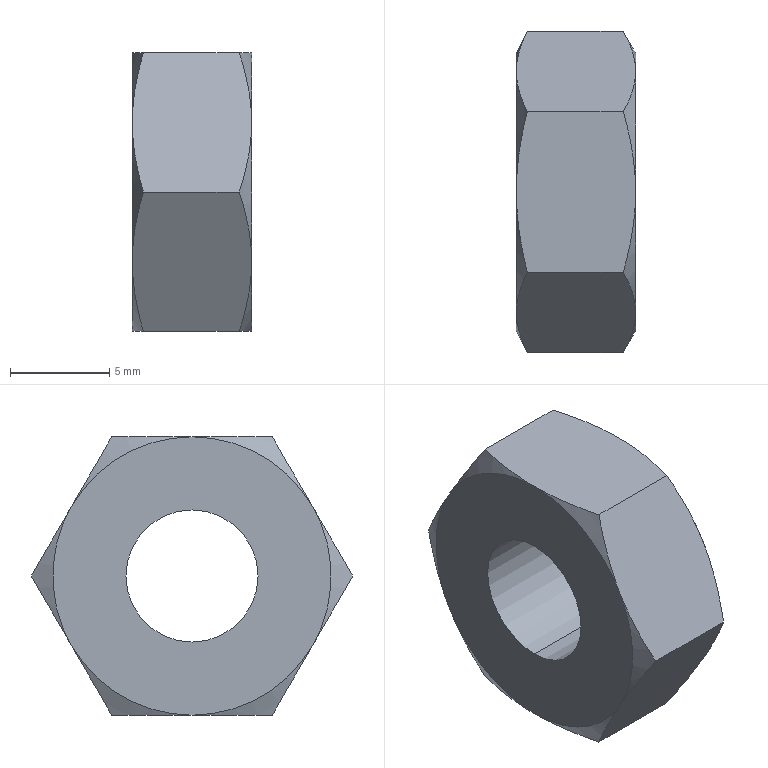Part | 1 solid | 22 faces | box 6 x 16.166 x 14 mm | volume 804.447 mm3 | cone 12 | plane 8 | cylinder 2 | commonest cylinder face diameters 6.647 x2
STEP:
#1=CARTESIAN_POINT('',(0.,0.,3.324));
#2=VERTEX_POINT('',#1);
#3=CARTESIAN_POINT('',(0.,0.,-3.324));
#4=VERTEX_POINT('',#3);
#5=CARTESIAN_POINT('',(0.,0.,0.));
#6=DIRECTION('',(1.,0.,0.));
#7=DIRECTION('',(0.,0.,-1.));
#8=AXIS2_PLACEMENT_3D('',#5,#6,#7);
#9=CIRCLE('',#8,3.324);
#10=EDGE_CURVE('',#2,#4,#9,.T.);
#11=ORIENTED_EDGE('',*,*,#10,.F.);
#12=CARTESIAN_POINT('',(6.,0.,3.324));
#13=VERTEX_POINT('',#12);
#14=CARTESIAN_POINT('',(6.,0.,3.324));
#15=DIRECTION('',(1.,0.,0.));
#16=VECTOR('',#15,1000.);
#17=LINE('',#14,#16);
#18=EDGE_CURVE('',#2,#13,#17,.T.);
#19=ORIENTED_EDGE('',*,*,#18,.T.);
#20=CARTESIAN_POINT('',(6.,0.,-3.324));
#21=VERTEX_POINT('',#20);
#22=CARTESIAN_POINT('',(6.,0.,0.));
#23=DIRECTION('',(1.,0.,0.));
#24=DIRECTION('',(0.,0.,-1.));
#25=AXIS2_PLACEMENT_3D('',#22,#23,#24);
#26=CIRCLE('',#25,3.324);
#27=EDGE_CURVE('',#13,#21,#26,.T.);
#28=ORIENTED_EDGE('',*,*,#27,.T.);
#29=CARTESIAN_POINT('',(6.,0.,-3.324));
#30=DIRECTION('',(1.,0.,0.));
#31=VECTOR('',#30,1000.);
#32=LINE('',#29,#31);
#33=EDGE_CURVE('',#4,#21,#32,.T.);
#34=ORIENTED_EDGE('',*,*,#33,.F.);
#35=EDGE_LOOP('',(#11,#19,#28,#34));
#36=FACE_OUTER_BOUND('',#35,.T.);
#37=CARTESIAN_POINT('',(6.,0.,0.));
#38=DIRECTION('',(1.,0.,0.));
#39=DIRECTION('',(0.,0.,-1.));
#40=AXIS2_PLACEMENT_3D('',#37,#38,#39);
#41=CYLINDRICAL_SURFACE('',#40,3.324);
#42=ADVANCED_FACE('',(#36),#41,.F.);
#43=CARTESIAN_POINT('',(5.375,-4.041,7.));
#44=VERTEX_POINT('',#43);
#45=CARTESIAN_POINT('',(6.,0.,7.));
#46=VERTEX_POINT('',#45);
#47=CARTESIAN_POINT('',(5.375,-4.041,7.));
#48=CARTESIAN_POINT('',(5.792,-2.598,7.));
#49=CARTESIAN_POINT('',(6.,-1.25,7.));
#50=CARTESIAN_POINT('',(6.,0.,7.));
#51=B_SPLINE_CURVE_WITH_KNOTS('',3,(#47,#48,#49,#50),.UNSPECIFIED.,.F.,.F.,(4,4),(0.,1.),.UNSPECIFIED.);
#52=EDGE_CURVE('',#44,#46,#51,.T.);
#53=ORIENTED_EDGE('',*,*,#52,.F.);
#54=CARTESIAN_POINT('',(6.,-6.062,3.5));
#55=VERTEX_POINT('',#54);
#56=CARTESIAN_POINT('',(6.,-6.062,3.5));
#57=CARTESIAN_POINT('',(6.,-5.437,4.583));
#58=CARTESIAN_POINT('',(5.792,-4.763,5.75));
#59=CARTESIAN_POINT('',(5.375,-4.041,7.));
#60=B_SPLINE_CURVE_WITH_KNOTS('',3,(#56,#57,#58,#59),.UNSPECIFIED.,.F.,.F.,(4,4),(0.,1.),.UNSPECIFIED.);
#61=EDGE_CURVE('',#55,#44,#60,.T.);
#62=ORIENTED_EDGE('',*,*,#61,.F.);
#63=CARTESIAN_POINT('',(6.,0.,0.));
#64=DIRECTION('',(1.,0.,0.));
#65=DIRECTION('',(0.,0.,-1.));
#66=AXIS2_PLACEMENT_3D('',#63,#64,#65);
#67=CIRCLE('',#66,7.);
#68=EDGE_CURVE('',#46,#55,#67,.T.);
#69=ORIENTED_EDGE('',*,*,#68,.F.);
#70=EDGE_LOOP('',(#53,#62,#69));
#71=FACE_OUTER_BOUND('',#70,.T.);
#72=CARTESIAN_POINT('',(6.,0.,0.));
#73=DIRECTION('',(-1.,0.,0.));
#74=DIRECTION('',(0.,0.,1.));
#75=AXIS2_PLACEMENT_3D('',#72,#73,#74);
#76=CONICAL_SURFACE('',#75,7.,1.047);
#77=ADVANCED_FACE('',(#71),#76,.T.);
#78=CARTESIAN_POINT('',(5.375,4.041,7.));
#79=VERTEX_POINT('',#78);
#80=CARTESIAN_POINT('',(6.,0.,7.));
#81=CARTESIAN_POINT('',(6.,1.25,7.));
#82=CARTESIAN_POINT('',(5.792,2.598,7.));
#83=CARTESIAN_POINT('',(5.375,4.041,7.));
#84=B_SPLINE_CURVE_WITH_KNOTS('',3,(#80,#81,#82,#83),.UNSPECIFIED.,.F.,.F.,(4,4),(0.,1.),.UNSPECIFIED.);
#85=EDGE_CURVE('',#46,#79,#84,.T.);
#86=ORIENTED_EDGE('',*,*,#85,.F.);
#87=CARTESIAN_POINT('',(6.,6.062,3.5));
#88=VERTEX_POINT('',#87);
#89=CARTESIAN_POINT('',(6.,0.,0.));
#90=DIRECTION('',(1.,0.,0.));
#91=DIRECTION('',(0.,0.,-1.));
#92=AXIS2_PLACEMENT_3D('',#89,#90,#91);
#93=CIRCLE('',#92,7.);
#94=EDGE_CURVE('',#88,#46,#93,.T.);
#95=ORIENTED_EDGE('',*,*,#94,.F.);
#96=CARTESIAN_POINT('',(5.375,4.041,7.));
#97=CARTESIAN_POINT('',(5.792,4.763,5.75));
#98=CARTESIAN_POINT('',(6.,5.437,4.583));
#99=CARTESIAN_POINT('',(6.,6.062,3.5));
#100=B_SPLINE_CURVE_WITH_KNOTS('',3,(#96,#97,#98,#99),.UNSPECIFIED.,.F.,.F.,(4,4),(0.,1.),.UNSPECIFIED.);
#101=EDGE_CURVE('',#79,#88,#100,.T.);
#102=ORIENTED_EDGE('',*,*,#101,.F.);
#103=EDGE_LOOP('',(#86,#95,#102));
#104=FACE_OUTER_BOUND('',#103,.T.);
#105=CARTESIAN_POINT('',(6.,0.,0.));
#106=DIRECTION('',(-1.,0.,0.));
#107=DIRECTION('',(0.,0.,1.));
#108=AXIS2_PLACEMENT_3D('',#105,#106,#107);
#109=CONICAL_SURFACE('',#108,7.,1.047);
#110=ADVANCED_FACE('',(#104),#109,.T.);
#111=CARTESIAN_POINT('',(5.375,8.083,0.));
#112=VERTEX_POINT('',#111);
#113=CARTESIAN_POINT('',(6.,6.062,3.5));
#114=CARTESIAN_POINT('',(6.,6.687,2.417));
#115=CARTESIAN_POINT('',(5.792,7.361,1.25));
#116=CARTESIAN_POINT('',(5.375,8.083,0.));
#117=B_SPLINE_CURVE_WITH_KNOTS('',3,(#113,#114,#115,#116),.UNSPECIFIED.,.F.,.F.,(4,4),(0.,1.),.UNSPECIFIED.);
#118=EDGE_CURVE('',#88,#112,#117,.T.);
#119=ORIENTED_EDGE('',*,*,#118,.F.);
#120=CARTESIAN_POINT('',(6.,6.062,-3.5));
#121=VERTEX_POINT('',#120);
#122=CARTESIAN_POINT('',(6.,0.,0.));
#123=DIRECTION('',(1.,0.,0.));
#124=DIRECTION('',(0.,0.,-1.));
#125=AXIS2_PLACEMENT_3D('',#122,#123,#124);
#126=CIRCLE('',#125,7.);
#127=EDGE_CURVE('',#121,#88,#126,.T.);
#128=ORIENTED_EDGE('',*,*,#127,.F.);
#129=CARTESIAN_POINT('',(5.375,8.083,0.));
#130=CARTESIAN_POINT('',(5.792,7.361,-1.25));
#131=CARTESIAN_POINT('',(6.,6.687,-2.417));
#132=CARTESIAN_POINT('',(6.,6.062,-3.5));
#133=B_SPLINE_CURVE_WITH_KNOTS('',3,(#129,#130,#131,#132),.UNSPECIFIED.,.F.,.F.,(4,4),(0.,1.),.UNSPECIFIED.);
#134=EDGE_CURVE('',#112,#121,#133,.T.);
#135=ORIENTED_EDGE('',*,*,#134,.F.);
#136=EDGE_LOOP('',(#119,#128,#135));
#137=FACE_OUTER_BOUND('',#136,.T.);
#138=CARTESIAN_POINT('',(6.,0.,0.));
#139=DIRECTION('',(-1.,0.,0.));
#140=DIRECTION('',(0.,0.,1.));
#141=AXIS2_PLACEMENT_3D('',#138,#139,#140);
#142=CONICAL_SURFACE('',#141,7.,1.047);
#143=ADVANCED_FACE('',(#137),#142,.T.);
#144=CARTESIAN_POINT('',(5.375,4.041,-7.));
#145=VERTEX_POINT('',#144);
#146=CARTESIAN_POINT('',(6.,6.062,-3.5));
#147=CARTESIAN_POINT('',(6.,5.437,-4.583));
#148=CARTESIAN_POINT('',(5.792,4.763,-5.75));
#149=CARTESIAN_POINT('',(5.375,4.041,-7.));
#150=B_SPLINE_CURVE_WITH_KNOTS('',3,(#146,#147,#148,#149),.UNSPECIFIED.,.F.,.F.,(4,4),(0.,1.),.UNSPECIFIED.);
#151=EDGE_CURVE('',#121,#145,#150,.T.);
#152=ORIENTED_EDGE('',*,*,#151,.F.);
#153=CARTESIAN_POINT('',(6.,0.,-7.));
#154=VERTEX_POINT('',#153);
#155=CARTESIAN_POINT('',(6.,0.,0.));
#156=DIRECTION('',(1.,0.,0.));
#157=DIRECTION('',(0.,0.,-1.));
#158=AXIS2_PLACEMENT_3D('',#155,#156,#157);
#159=CIRCLE('',#158,7.);
#160=EDGE_CURVE('',#154,#121,#159,.T.);
#161=ORIENTED_EDGE('',*,*,#160,.F.);
#162=CARTESIAN_POINT('',(5.375,4.041,-7.));
#163=CARTESIAN_POINT('',(5.792,2.598,-7.));
#164=CARTESIAN_POINT('',(6.,1.25,-7.));
#165=CARTESIAN_POINT('',(6.,0.,-7.));
#166=B_SPLINE_CURVE_WITH_KNOTS('',3,(#162,#163,#164,#165),.UNSPECIFIED.,.F.,.F.,(4,4),(0.,1.),.UNSPECIFIED.);
#167=EDGE_CURVE('',#145,#154,#166,.T.);
#168=ORIENTED_EDGE('',*,*,#167,.F.);
#169=EDGE_LOOP('',(#152,#161,#168));
#170=FACE_OUTER_BOUND('',#169,.T.);
#171=CARTESIAN_POINT('',(6.,0.,0.));
#172=DIRECTION('',(-1.,0.,0.));
#173=DIRECTION('',(0.,0.,1.));
#174=AXIS2_PLACEMENT_3D('',#171,#172,#173);
#175=CONICAL_SURFACE('',#174,7.,1.047);
#176=ADVANCED_FACE('',(#170),#175,.T.);
#177=CARTESIAN_POINT('',(5.375,-4.041,-7.));
#178=VERTEX_POINT('',#177);
#179=CARTESIAN_POINT('',(6.,0.,-7.));
#180=CARTESIAN_POINT('',(6.,-1.25,-7.));
#181=CARTESIAN_POINT('',(5.792,-2.598,-7.));
#182=CARTESIAN_POINT('',(5.375,-4.041,-7.));
#183=B_SPLINE_CURVE_WITH_KNOTS('',3,(#179,#180,#181,#182),.UNSPECIFIED.,.F.,.F.,(4,4),(0.,1.),.UNSPECIFIED.);
#184=EDGE_CURVE('',#154,#178,#183,.T.);
#185=ORIENTED_EDGE('',*,*,#184,.F.);
#186=CARTESIAN_POINT('',(6.,-6.062,-3.5));
#187=VERTEX_POINT('',#186);
#188=CARTESIAN_POINT('',(6.,0.,0.));
#189=DIRECTION('',(1.,0.,0.));
#190=DIRECTION('',(0.,0.,-1.));
#191=AXIS2_PLACEMENT_3D('',#188,#189,#190);
#192=CIRCLE('',#191,7.);
#193=EDGE_CURVE('',#187,#154,#192,.T.);
#194=ORIENTED_EDGE('',*,*,#193,.F.);
#195=CARTESIAN_POINT('',(5.375,-4.041,-7.));
#196=CARTESIAN_POINT('',(5.792,-4.763,-5.75));
#197=CARTESIAN_POINT('',(6.,-5.437,-4.583));
#198=CARTESIAN_POINT('',(6.,-6.062,-3.5));
#199=B_SPLINE_CURVE_WITH_KNOTS('',3,(#195,#196,#197,#198),.UNSPECIFIED.,.F.,.F.,(4,4),(0.,1.),.UNSPECIFIED.);
#200=EDGE_CURVE('',#178,#187,#199,.T.);
#201=ORIENTED_EDGE('',*,*,#200,.F.);
#202=EDGE_LOOP('',(#185,#194,#201));
#203=FACE_OUTER_BOUND('',#202,.T.);
#204=CARTESIAN_POINT('',(6.,0.,0.));
#205=DIRECTION('',(-1.,0.,0.));
#206=DIRECTION('',(0.,0.,1.));
#207=AXIS2_PLACEMENT_3D('',#204,#205,#206);
#208=CONICAL_SURFACE('',#207,7.,1.047);
#209=ADVANCED_FACE('',(#203),#208,.T.);
#210=CARTESIAN_POINT('',(0.5518,4.041,-7.));
#211=VERTEX_POINT('',#210);
#212=CARTESIAN_POINT('',(0.,6.062,-3.5));
#213=VERTEX_POINT('',#212);
#214=CARTESIAN_POINT('',(0.5518,4.041,-7.));
#215=CARTESIAN_POINT('',(0.1839,4.763,-5.75));
#216=CARTESIAN_POINT('',(0.,5.437,-4.583));
#217=CARTESIAN_POINT('',(0.,6.062,-3.5));
#218=B_SPLINE_CURVE_WITH_KNOTS('',3,(#214,#215,#216,#217),.UNSPECIFIED.,.F.,.F.,(4,4),(0.,1.),.UNSPECIFIED.);
#219=EDGE_CURVE('',#211,#213,#218,.T.);
#220=ORIENTED_EDGE('',*,*,#219,.F.);
#221=CARTESIAN_POINT('',(0.,0.,-7.));
#222=VERTEX_POINT('',#221);
#223=CARTESIAN_POINT('',(0.,0.,-7.));
#224=CARTESIAN_POINT('',(0.,1.25,-7.));
#225=CARTESIAN_POINT('',(0.1839,2.598,-7.));
#226=CARTESIAN_POINT('',(0.5518,4.041,-7.));
#227=B_SPLINE_CURVE_WITH_KNOTS('',3,(#223,#224,#225,#226),.UNSPECIFIED.,.F.,.F.,(4,4),(0.,1.),.UNSPECIFIED.);
#228=EDGE_CURVE('',#222,#211,#227,.T.);
#229=ORIENTED_EDGE('',*,*,#228,.F.);
#230=CARTESIAN_POINT('',(0.,0.,0.));
#231=DIRECTION('',(1.,0.,0.));
#232=DIRECTION('',(0.,0.,-1.));
#233=AXIS2_PLACEMENT_3D('',#230,#231,#232);
#234=CIRCLE('',#233,7.);
#235=EDGE_CURVE('',#222,#213,#234,.T.);
#236=ORIENTED_EDGE('',*,*,#235,.T.);
#237=EDGE_LOOP('',(#220,#229,#236));
#238=FACE_OUTER_BOUND('',#237,.T.);
#239=CARTESIAN_POINT('',(2.813,0.,0.));
#240=DIRECTION('',(1.,0.,0.));
#241=DIRECTION('',(0.,0.,-1.));
#242=AXIS2_PLACEMENT_3D('',#239,#240,#241);
#243=CONICAL_SURFACE('',#242,12.52,1.1);
#244=ADVANCED_FACE('',(#238),#243,.T.);
#245=CARTESIAN_POINT('',(0.5518,8.083,0.));
#246=VERTEX_POINT('',#245);
#247=CARTESIAN_POINT('',(0.,6.062,-3.5));
#248=CARTESIAN_POINT('',(0.,6.687,-2.417));
#249=CARTESIAN_POINT('',(0.1839,7.361,-1.25));
#250=CARTESIAN_POINT('',(0.5518,8.083,0.));
#251=B_SPLINE_CURVE_WITH_KNOTS('',3,(#247,#248,#249,#250),.UNSPECIFIED.,.F.,.F.,(4,4),(0.,1.),.UNSPECIFIED.);
#252=EDGE_CURVE('',#213,#246,#251,.T.);
#253=ORIENTED_EDGE('',*,*,#252,.F.);
#254=CARTESIAN_POINT('',(0.,6.062,3.5));
#255=VERTEX_POINT('',#254);
#256=CARTESIAN_POINT('',(0.,0.,0.));
#257=DIRECTION('',(1.,0.,0.));
#258=DIRECTION('',(0.,0.,-1.));
#259=AXIS2_PLACEMENT_3D('',#256,#257,#258);
#260=CIRCLE('',#259,7.);
#261=EDGE_CURVE('',#213,#255,#260,.T.);
#262=ORIENTED_EDGE('',*,*,#261,.T.);
#263=CARTESIAN_POINT('',(0.5518,8.083,0.));
#264=CARTESIAN_POINT('',(0.1839,7.361,1.25));
#265=CARTESIAN_POINT('',(0.,6.687,2.417));
#266=CARTESIAN_POINT('',(0.,6.062,3.5));
#267=B_SPLINE_CURVE_WITH_KNOTS('',3,(#263,#264,#265,#266),.UNSPECIFIED.,.F.,.F.,(4,4),(0.,1.),.UNSPECIFIED.);
#268=EDGE_CURVE('',#246,#255,#267,.T.);
#269=ORIENTED_EDGE('',*,*,#268,.F.);
#270=EDGE_LOOP('',(#253,#262,#269));
#271=FACE_OUTER_BOUND('',#270,.T.);
#272=CARTESIAN_POINT('',(2.813,0.,0.));
#273=DIRECTION('',(1.,0.,0.));
#274=DIRECTION('',(0.,0.,-1.));
#275=AXIS2_PLACEMENT_3D('',#272,#273,#274);
#276=CONICAL_SURFACE('',#275,12.52,1.1);
#277=ADVANCED_FACE('',(#271),#276,.T.);
#278=CARTESIAN_POINT('',(0.5518,4.041,7.));
#279=VERTEX_POINT('',#278);
#280=CARTESIAN_POINT('',(0.,6.062,3.5));
#281=CARTESIAN_POINT('',(0.,5.437,4.583));
#282=CARTESIAN_POINT('',(0.1839,4.763,5.75));
#283=CARTESIAN_POINT('',(0.5518,4.041,7.));
#284=B_SPLINE_CURVE_WITH_KNOTS('',3,(#280,#281,#282,#283),.UNSPECIFIED.,.F.,.F.,(4,4),(0.,1.),.UNSPECIFIED.);
#285=EDGE_CURVE('',#255,#279,#284,.T.);
#286=ORIENTED_EDGE('',*,*,#285,.F.);
#287=CARTESIAN_POINT('',(0.,0.,7.));
#288=VERTEX_POINT('',#287);
#289=CARTESIAN_POINT('',(0.,0.,0.));
#290=DIRECTION('',(1.,0.,0.));
#291=DIRECTION('',(0.,0.,-1.));
#292=AXIS2_PLACEMENT_3D('',#289,#290,#291);
#293=CIRCLE('',#292,7.);
#294=EDGE_CURVE('',#255,#288,#293,.T.);
#295=ORIENTED_EDGE('',*,*,#294,.T.);
#296=CARTESIAN_POINT('',(0.5518,4.041,7.));
#297=CARTESIAN_POINT('',(0.1839,2.598,7.));
#298=CARTESIAN_POINT('',(0.,1.25,7.));
#299=CARTESIAN_POINT('',(0.,0.,7.));
#300=B_SPLINE_CURVE_WITH_KNOTS('',3,(#296,#297,#298,#299),.UNSPECIFIED.,.F.,.F.,(4,4),(0.,1.),.UNSPECIFIED.);
#301=EDGE_CURVE('',#279,#288,#300,.T.);
#302=ORIENTED_EDGE('',*,*,#301,.F.);
#303=EDGE_LOOP('',(#286,#295,#302));
#304=FACE_OUTER_BOUND('',#303,.T.);
#305=CARTESIAN_POINT('',(2.813,0.,0.));
#306=DIRECTION('',(1.,0.,0.));
#307=DIRECTION('',(0.,0.,-1.));
#308=AXIS2_PLACEMENT_3D('',#305,#306,#307);
#309=CONICAL_SURFACE('',#308,12.52,1.1);
#310=ADVANCED_FACE('',(#304),#309,.T.);
#311=CARTESIAN_POINT('',(0.5518,-4.041,-7.));
#312=VERTEX_POINT('',#311);
#313=CARTESIAN_POINT('',(0.5518,-4.041,-7.));
#314=CARTESIAN_POINT('',(0.1839,-2.598,-7.));
#315=CARTESIAN_POINT('',(0.,-1.25,-7.));
#316=CARTESIAN_POINT('',(0.,0.,-7.));
#317=B_SPLINE_CURVE_WITH_KNOTS('',3,(#313,#314,#315,#316),.UNSPECIFIED.,.F.,.F.,(4,4),(0.,1.),.UNSPECIFIED.);
#318=EDGE_CURVE('',#312,#222,#317,.T.);
#319=ORIENTED_EDGE('',*,*,#318,.F.);
#320=CARTESIAN_POINT('',(0.,-6.062,-3.5));
#321=VERTEX_POINT('',#320);
#322=CARTESIAN_POINT('',(0.,-6.062,-3.5));
#323=CARTESIAN_POINT('',(0.,-5.437,-4.583));
#324=CARTESIAN_POINT('',(0.1839,-4.763,-5.75));
#325=CARTESIAN_POINT('',(0.5518,-4.041,-7.));
#326=B_SPLINE_CURVE_WITH_KNOTS('',3,(#322,#323,#324,#325),.UNSPECIFIED.,.F.,.F.,(4,4),(0.,1.),.UNSPECIFIED.);
#327=EDGE_CURVE('',#321,#312,#326,.T.);
#328=ORIENTED_EDGE('',*,*,#327,.F.);
#329=CARTESIAN_POINT('',(0.,0.,0.));
#330=DIRECTION('',(1.,0.,0.));
#331=DIRECTION('',(0.,0.,-1.));
#332=AXIS2_PLACEMENT_3D('',#329,#330,#331);
#333=CIRCLE('',#332,7.);
#334=EDGE_CURVE('',#321,#222,#333,.T.);
#335=ORIENTED_EDGE('',*,*,#334,.T.);
#336=EDGE_LOOP('',(#319,#328,#335));
#337=FACE_OUTER_BOUND('',#336,.T.);
#338=CARTESIAN_POINT('',(2.813,0.,0.));
#339=DIRECTION('',(1.,0.,0.));
#340=DIRECTION('',(0.,0.,-1.));
#341=AXIS2_PLACEMENT_3D('',#338,#339,#340);
#342=CONICAL_SURFACE('',#341,12.52,1.1);
#343=ADVANCED_FACE('',(#337),#342,.T.);
#344=CARTESIAN_POINT('',(0.5518,-4.041,7.));
#345=VERTEX_POINT('',#344);
#346=CARTESIAN_POINT('',(0.,0.,7.));
#347=CARTESIAN_POINT('',(0.,-1.25,7.));
#348=CARTESIAN_POINT('',(0.1839,-2.598,7.));
#349=CARTESIAN_POINT('',(0.5518,-4.041,7.));
#350=B_SPLINE_CURVE_WITH_KNOTS('',3,(#346,#347,#348,#349),.UNSPECIFIED.,.F.,.F.,(4,4),(0.,1.),.UNSPECIFIED.);
#351=EDGE_CURVE('',#288,#345,#350,.T.);
#352=ORIENTED_EDGE('',*,*,#351,.F.);
#353=CARTESIAN_POINT('',(0.,-6.062,3.5));
#354=VERTEX_POINT('',#353);
#355=CARTESIAN_POINT('',(0.,0.,0.));
#356=DIRECTION('',(1.,0.,0.));
#357=DIRECTION('',(0.,0.,-1.));
#358=AXIS2_PLACEMENT_3D('',#355,#356,#357);
#359=CIRCLE('',#358,7.);
#360=EDGE_CURVE('',#288,#354,#359,.T.);
#361=ORIENTED_EDGE('',*,*,#360,.T.);
#362=CARTESIAN_POINT('',(0.5518,-4.041,7.));
#363=CARTESIAN_POINT('',(0.1839,-4.763,5.75));
#364=CARTESIAN_POINT('',(0.,-5.437,4.583));
#365=CARTESIAN_POINT('',(0.,-6.062,3.5));
#366=B_SPLINE_CURVE_WITH_KNOTS('',3,(#362,#363,#364,#365),.UNSPECIFIED.,.F.,.F.,(4,4),(0.,1.),.UNSPECIFIED.);
#367=EDGE_CURVE('',#345,#354,#366,.T.);
#368=ORIENTED_EDGE('',*,*,#367,.F.);
#369=EDGE_LOOP('',(#352,#361,#368));
#370=FACE_OUTER_BOUND('',#369,.T.);
#371=CARTESIAN_POINT('',(2.813,0.,0.));
#372=DIRECTION('',(1.,0.,0.));
#373=DIRECTION('',(0.,0.,-1.));
#374=AXIS2_PLACEMENT_3D('',#371,#372,#373);
#375=CONICAL_SURFACE('',#374,12.52,1.1);
#376=ADVANCED_FACE('',(#370),#375,.T.);
#377=CARTESIAN_POINT('',(0.,0.,0.));
#378=DIRECTION('',(1.,0.,0.));
#379=DIRECTION('',(0.,0.,-1.));
#380=AXIS2_PLACEMENT_3D('',#377,#378,#379);
#381=CIRCLE('',#380,3.324);
#382=EDGE_CURVE('',#4,#2,#381,.T.);
#383=ORIENTED_EDGE('',*,*,#382,.T.);
#384=ORIENTED_EDGE('',*,*,#10,.T.);
#385=EDGE_LOOP('',(#383,#384));
#386=FACE_BOUND('',#385,.T.);
#387=ORIENTED_EDGE('',*,*,#235,.F.);
#388=ORIENTED_EDGE('',*,*,#334,.F.);
#389=CARTESIAN_POINT('',(0.,0.,0.));
#390=DIRECTION('',(1.,0.,0.));
#391=DIRECTION('',(0.,0.,-1.));
#392=AXIS2_PLACEMENT_3D('',#389,#390,#391);
#393=CIRCLE('',#392,7.);
#394=EDGE_CURVE('',#354,#321,#393,.T.);
#395=ORIENTED_EDGE('',*,*,#394,.F.);
#396=ORIENTED_EDGE('',*,*,#360,.F.);
#397=ORIENTED_EDGE('',*,*,#294,.F.);
#398=ORIENTED_EDGE('',*,*,#261,.F.);
#399=EDGE_LOOP('',(#387,#388,#395,#396,#397,#398));
#400=FACE_OUTER_BOUND('',#399,.T.);
#401=CARTESIAN_POINT('',(0.,7.,0.));
#402=DIRECTION('',(-1.,0.,0.));
#403=DIRECTION('',(0.,0.,1.));
#404=AXIS2_PLACEMENT_3D('',#401,#402,#403);
#405=PLANE('',#404);
#406=ADVANCED_FACE('',(#386,#400),#405,.T.);
#407=ORIENTED_EDGE('',*,*,#18,.F.);
#408=ORIENTED_EDGE('',*,*,#382,.F.);
#409=ORIENTED_EDGE('',*,*,#33,.T.);
#410=CARTESIAN_POINT('',(6.,0.,0.));
#411=DIRECTION('',(1.,0.,0.));
#412=DIRECTION('',(0.,0.,-1.));
#413=AXIS2_PLACEMENT_3D('',#410,#411,#412);
#414=CIRCLE('',#413,3.324);
#415=EDGE_CURVE('',#21,#13,#414,.T.);
#416=ORIENTED_EDGE('',*,*,#415,.T.);
#417=EDGE_LOOP('',(#407,#408,#409,#416));
#418=FACE_OUTER_BOUND('',#417,.T.);
#419=CARTESIAN_POINT('',(6.,0.,0.));
#420=DIRECTION('',(1.,0.,0.));
#421=DIRECTION('',(0.,0.,-1.));
#422=AXIS2_PLACEMENT_3D('',#419,#420,#421);
#423=CYLINDRICAL_SURFACE('',#422,3.324);
#424=ADVANCED_FACE('',(#418),#423,.F.);
#425=ORIENTED_EDGE('',*,*,#160,.T.);
#426=ORIENTED_EDGE('',*,*,#127,.T.);
#427=ORIENTED_EDGE('',*,*,#94,.T.);
#428=ORIENTED_EDGE('',*,*,#68,.T.);
#429=CARTESIAN_POINT('',(6.,0.,0.));
#430=DIRECTION('',(1.,0.,0.));
#431=DIRECTION('',(0.,0.,-1.));
#432=AXIS2_PLACEMENT_3D('',#429,#430,#431);
#433=CIRCLE('',#432,7.);
#434=EDGE_CURVE('',#55,#187,#433,.T.);
#435=ORIENTED_EDGE('',*,*,#434,.T.);
#436=ORIENTED_EDGE('',*,*,#193,.T.);
#437=EDGE_LOOP('',(#425,#426,#427,#428,#435,#436));
#438=FACE_OUTER_BOUND('',#437,.T.);
#439=ORIENTED_EDGE('',*,*,#415,.F.);
#440=ORIENTED_EDGE('',*,*,#27,.F.);
#441=EDGE_LOOP('',(#439,#440));
#442=FACE_BOUND('',#441,.T.);
#443=CARTESIAN_POINT('',(6.,3.324,0.));
#444=DIRECTION('',(1.,0.,0.));
#445=DIRECTION('',(0.,1.,0.));
#446=AXIS2_PLACEMENT_3D('',#443,#444,#445);
#447=PLANE('',#446);
#448=ADVANCED_FACE('',(#438,#442),#447,.T.);
#449=CARTESIAN_POINT('',(5.375,-8.083,0.));
#450=VERTEX_POINT('',#449);
#451=CARTESIAN_POINT('',(6.,-6.062,-3.5));
#452=CARTESIAN_POINT('',(6.,-6.687,-2.417));
#453=CARTESIAN_POINT('',(5.792,-7.361,-1.25));
#454=CARTESIAN_POINT('',(5.375,-8.083,0.));
#455=B_SPLINE_CURVE_WITH_KNOTS('',3,(#451,#452,#453,#454),.UNSPECIFIED.,.F.,.F.,(4,4),(0.,1.),.UNSPECIFIED.);
#456=EDGE_CURVE('',#187,#450,#455,.T.);
#457=ORIENTED_EDGE('',*,*,#456,.F.);
#458=ORIENTED_EDGE('',*,*,#434,.F.);
#459=CARTESIAN_POINT('',(5.375,-8.083,0.));
#460=CARTESIAN_POINT('',(5.792,-7.361,1.25));
#461=CARTESIAN_POINT('',(6.,-6.687,2.417));
#462=CARTESIAN_POINT('',(6.,-6.062,3.5));
#463=B_SPLINE_CURVE_WITH_KNOTS('',3,(#459,#460,#461,#462),.UNSPECIFIED.,.F.,.F.,(4,4),(0.,1.),.UNSPECIFIED.);
#464=EDGE_CURVE('',#450,#55,#463,.T.);
#465=ORIENTED_EDGE('',*,*,#464,.F.);
#466=EDGE_LOOP('',(#457,#458,#465));
#467=FACE_OUTER_BOUND('',#466,.T.);
#468=CARTESIAN_POINT('',(6.,0.,0.));
#469=DIRECTION('',(-1.,0.,0.));
#470=DIRECTION('',(0.,0.,1.));
#471=AXIS2_PLACEMENT_3D('',#468,#469,#470);
#472=CONICAL_SURFACE('',#471,7.,1.047);
#473=ADVANCED_FACE('',(#467),#472,.T.);
#474=CARTESIAN_POINT('',(0.5518,-8.083,0.));
#475=VERTEX_POINT('',#474);
#476=CARTESIAN_POINT('',(0.5518,-8.083,0.));
#477=CARTESIAN_POINT('',(0.1839,-7.361,-1.25));
#478=CARTESIAN_POINT('',(0.,-6.687,-2.417));
#479=CARTESIAN_POINT('',(0.,-6.062,-3.5));
#480=B_SPLINE_CURVE_WITH_KNOTS('',3,(#476,#477,#478,#479),.UNSPECIFIED.,.F.,.F.,(4,4),(0.,1.),.UNSPECIFIED.);
#481=EDGE_CURVE('',#475,#321,#480,.T.);
#482=ORIENTED_EDGE('',*,*,#481,.F.);
#483=CARTESIAN_POINT('',(0.,-6.062,3.5));
#484=CARTESIAN_POINT('',(0.,-6.687,2.417));
#485=CARTESIAN_POINT('',(0.1839,-7.361,1.25));
#486=CARTESIAN_POINT('',(0.5518,-8.083,0.));
#487=B_SPLINE_CURVE_WITH_KNOTS('',3,(#483,#484,#485,#486),.UNSPECIFIED.,.F.,.F.,(4,4),(0.,1.),.UNSPECIFIED.);
#488=EDGE_CURVE('',#354,#475,#487,.T.);
#489=ORIENTED_EDGE('',*,*,#488,.F.);
#490=ORIENTED_EDGE('',*,*,#394,.T.);
#491=EDGE_LOOP('',(#482,#489,#490));
#492=FACE_OUTER_BOUND('',#491,.T.);
#493=CARTESIAN_POINT('',(2.813,0.,0.));
#494=DIRECTION('',(1.,0.,0.));
#495=DIRECTION('',(0.,0.,-1.));
#496=AXIS2_PLACEMENT_3D('',#493,#494,#495);
#497=CONICAL_SURFACE('',#496,12.52,1.1);
#498=ADVANCED_FACE('',(#492),#497,.T.);
#499=ORIENTED_EDGE('',*,*,#52,.T.);
#500=ORIENTED_EDGE('',*,*,#85,.T.);
#501=CARTESIAN_POINT('',(6.,4.041,7.));
#502=DIRECTION('',(-1.,0.,0.));
#503=VECTOR('',#502,1000.);
#504=LINE('',#501,#503);
#505=EDGE_CURVE('',#79,#279,#504,.T.);
#506=ORIENTED_EDGE('',*,*,#505,.T.);
#507=ORIENTED_EDGE('',*,*,#301,.T.);
#508=ORIENTED_EDGE('',*,*,#351,.T.);
#509=CARTESIAN_POINT('',(6.,-4.041,7.));
#510=DIRECTION('',(-1.,0.,0.));
#511=VECTOR('',#510,1000.);
#512=LINE('',#509,#511);
#513=EDGE_CURVE('',#44,#345,#512,.T.);
#514=ORIENTED_EDGE('',*,*,#513,.F.);
#515=EDGE_LOOP('',(#499,#500,#506,#507,#508,#514));
#516=FACE_OUTER_BOUND('',#515,.T.);
#517=CARTESIAN_POINT('',(6.,4.041,7.));
#518=DIRECTION('',(0.,0.,-1.));
#519=DIRECTION('',(0.,-1.,0.));
#520=AXIS2_PLACEMENT_3D('',#517,#518,#519);
#521=PLANE('',#520);
#522=ADVANCED_FACE('',(#516),#521,.F.);
#523=ORIENTED_EDGE('',*,*,#101,.T.);
#524=ORIENTED_EDGE('',*,*,#118,.T.);
#525=CARTESIAN_POINT('',(6.,8.083,0.));
#526=DIRECTION('',(-1.,0.,0.));
#527=VECTOR('',#526,1000.);
#528=LINE('',#525,#527);
#529=EDGE_CURVE('',#112,#246,#528,.T.);
#530=ORIENTED_EDGE('',*,*,#529,.T.);
#531=ORIENTED_EDGE('',*,*,#268,.T.);
#532=ORIENTED_EDGE('',*,*,#285,.T.);
#533=ORIENTED_EDGE('',*,*,#505,.F.);
#534=EDGE_LOOP('',(#523,#524,#530,#531,#532,#533));
#535=FACE_OUTER_BOUND('',#534,.T.);
#536=CARTESIAN_POINT('',(6.,8.083,0.));
#537=DIRECTION('',(0.,-0.866,-0.5));
#538=DIRECTION('',(0.,0.5,-0.866));
#539=AXIS2_PLACEMENT_3D('',#536,#537,#538);
#540=PLANE('',#539);
#541=ADVANCED_FACE('',(#535),#540,.F.);
#542=ORIENTED_EDGE('',*,*,#134,.T.);
#543=ORIENTED_EDGE('',*,*,#151,.T.);
#544=CARTESIAN_POINT('',(6.,4.041,-7.));
#545=DIRECTION('',(-1.,0.,0.));
#546=VECTOR('',#545,1000.);
#547=LINE('',#544,#546);
#548=EDGE_CURVE('',#145,#211,#547,.T.);
#549=ORIENTED_EDGE('',*,*,#548,.T.);
#550=ORIENTED_EDGE('',*,*,#219,.T.);
#551=ORIENTED_EDGE('',*,*,#252,.T.);
#552=ORIENTED_EDGE('',*,*,#529,.F.);
#553=EDGE_LOOP('',(#542,#543,#549,#550,#551,#552));
#554=FACE_OUTER_BOUND('',#553,.T.);
#555=CARTESIAN_POINT('',(6.,4.041,-7.));
#556=DIRECTION('',(0.,-0.866,0.5));
#557=DIRECTION('',(-1.,0.,0.));
#558=AXIS2_PLACEMENT_3D('',#555,#556,#557);
#559=PLANE('',#558);
#560=ADVANCED_FACE('',(#554),#559,.F.);
#561=ORIENTED_EDGE('',*,*,#167,.T.);
#562=ORIENTED_EDGE('',*,*,#184,.T.);
#563=CARTESIAN_POINT('',(6.,-4.041,-7.));
#564=DIRECTION('',(-1.,0.,0.));
#565=VECTOR('',#564,1000.);
#566=LINE('',#563,#565);
#567=EDGE_CURVE('',#178,#312,#566,.T.);
#568=ORIENTED_EDGE('',*,*,#567,.T.);
#569=ORIENTED_EDGE('',*,*,#318,.T.);
#570=ORIENTED_EDGE('',*,*,#228,.T.);
#571=ORIENTED_EDGE('',*,*,#548,.F.);
#572=EDGE_LOOP('',(#561,#562,#568,#569,#570,#571));
#573=FACE_OUTER_BOUND('',#572,.T.);
#574=CARTESIAN_POINT('',(6.,-4.041,-7.));
#575=DIRECTION('',(0.,0.,1.));
#576=DIRECTION('',(1.,0.,0.));
#577=AXIS2_PLACEMENT_3D('',#574,#575,#576);
#578=PLANE('',#577);
#579=ADVANCED_FACE('',(#573),#578,.F.);
#580=ORIENTED_EDGE('',*,*,#200,.T.);
#581=ORIENTED_EDGE('',*,*,#456,.T.);
#582=CARTESIAN_POINT('',(6.,-8.083,0.));
#583=DIRECTION('',(-1.,0.,0.));
#584=VECTOR('',#583,1000.);
#585=LINE('',#582,#584);
#586=EDGE_CURVE('',#450,#475,#585,.T.);
#587=ORIENTED_EDGE('',*,*,#586,.T.);
#588=ORIENTED_EDGE('',*,*,#481,.T.);
#589=ORIENTED_EDGE('',*,*,#327,.T.);
#590=ORIENTED_EDGE('',*,*,#567,.F.);
#591=EDGE_LOOP('',(#580,#581,#587,#588,#589,#590));
#592=FACE_OUTER_BOUND('',#591,.T.);
#593=CARTESIAN_POINT('',(6.,-8.083,0.));
#594=DIRECTION('',(0.,0.866,0.5));
#595=DIRECTION('',(1.,0.,0.));
#596=AXIS2_PLACEMENT_3D('',#593,#594,#595);
#597=PLANE('',#596);
#598=ADVANCED_FACE('',(#592),#597,.F.);
#599=ORIENTED_EDGE('',*,*,#464,.T.);
#600=ORIENTED_EDGE('',*,*,#61,.T.);
#601=ORIENTED_EDGE('',*,*,#513,.T.);
#602=ORIENTED_EDGE('',*,*,#367,.T.);
#603=ORIENTED_EDGE('',*,*,#488,.T.);
#604=ORIENTED_EDGE('',*,*,#586,.F.);
#605=EDGE_LOOP('',(#599,#600,#601,#602,#603,#604));
#606=FACE_OUTER_BOUND('',#605,.T.);
#607=CARTESIAN_POINT('',(6.,-4.041,7.));
#608=DIRECTION('',(0.,0.866,-0.5));
#609=DIRECTION('',(-1.,0.,0.));
#610=AXIS2_PLACEMENT_3D('',#607,#608,#609);
#611=PLANE('',#610);
#612=ADVANCED_FACE('',(#606),#611,.F.);
#613=CLOSED_SHELL('',(#42,#77,#110,#143,#176,#209,#244,#277,#310,#343,#376,#406,#424,#448,#473,#498,#522,#541,#560,#579,#598,#612));
#614=MANIFOLD_SOLID_BREP('',#613);
#615=CARTESIAN_POINT('',(0.,0.,0.));
#616=DIRECTION('',(0.,0.,1.));
#617=DIRECTION('',(1.,0.,0.));
#618=AXIS2_PLACEMENT_3D('',#615,#616,#617);
#619=(LENGTH_UNIT()NAMED_UNIT(*)SI_UNIT(.MILLI.,.METRE.));
#620=UNCERTAINTY_MEASURE_WITH_UNIT(LENGTH_MEASURE(0.00001),#619,'','');
#621=(NAMED_UNIT(*)PLANE_ANGLE_UNIT()SI_UNIT($,.RADIAN.));
#622=(NAMED_UNIT(*)SI_UNIT($,.STERADIAN.)SOLID_ANGLE_UNIT());
#623=(GEOMETRIC_REPRESENTATION_CONTEXT(3)GLOBAL_UNCERTAINTY_ASSIGNED_CONTEXT((#620))GLOBAL_UNIT_ASSIGNED_CONTEXT((#619,#621,#622))REPRESENTATION_CONTEXT('',''));
#624=ADVANCED_BREP_SHAPE_REPRESENTATION('',(#614,#618),#623);